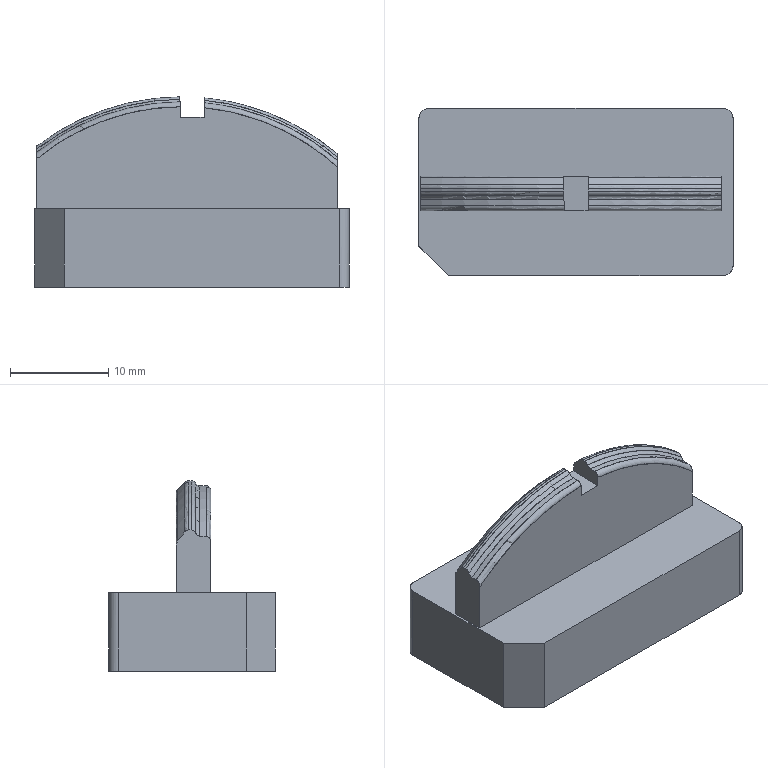NC program | PowerMill | posted with a generic post | part box 32 x 17 x 19.383 mm
Lines 1 to 1031 of 94163:
%
O0001
N104 ( POWERMILL CB  : 2026004.0)
N105 ( POST VER      : 2026.0.0.5161)
N106 ( OPTION FILE   : FANUC)
N107 ( OUTPUT WORKPLANE : WORLD)
N108 (  )
N109 ( TOOL LIST )
N110 (---------------------------------------)
N111 ( NO. | ID        | DIA.| TIP RAD|LENGTH)
N112 (---------------------------------------)
N113 (    1|D10C_1_1_1 |10.0 |  0.0   |74.84 )
N114 (    2|D4C_1_1    | 4.0 |  0.0   |66.56 )
N115 (   28|D2C_1_1    | 2.0 |  0.0   |57.36 )
N116 (    3|D10_1_1_1  |10.0 |  0.0   |74.56 )
N117 (   22|R1.5_1_1   | 3.0 |  1.5   | 64.0 )
N118 (    6|R0.5_1_1   | 1.0 |  0.5   |62.08 )
N119 (   12|D2_1_1     | 2.0 |  0.0   |57.48 )
N120 (   13|TEXT_D4_1_1| 4.0 |  0.3   |66.64 )
N121 (---------------------------------------)
N122 (  )
N123 ( NUMBER OF TOOLPATHS: 12.0 )
N124 ( ESTIMATED PROGRAM DURATION: 0 HOURS 8 MIN 19 SEC)
N125 (  )
N126 G00 G21 G80 G40 G17
N127 G90
N128 G54
N129 G53 Z0.0
N130 (---------------)
N131 ( START TOOLPATH : 精公开粗01-扫面平行-D10C )
N132 (---------------)
N133 ( TOOL NO.    :1 )
N134 ( TOOL TYPE   : ENDMILL)
N135 ( TOOL ID     : D10C_1_1_1)
N136 ( TOOL DIA    : 10.0 LENGTH 74.84)
N137 T1
N138 M6
N139 S8000 M03
N140 G00 G90 X0.0 Y0.0
N141 G43 Z10.2 H1
N142
N143 G05 P10000 R4
N144 X23.78 Y11.28
N145 Z1.133
N146 G01 Z-0.067 F6000.0
N147 X18.78 F10000.0
N148 X-18.78
N149 Y5.64
N150 X18.78
N151 Y0.0
N152 X-18.78
N153 Y-5.64
N154 X18.78
N155 Y-11.28
N156 X-18.78
N157 X-23.78
N158 G00 Z10.2
N159 G05 P0
N160 (---------------)
N161 ( END TOOLPATH : 精公开粗01-扫面平行-D10C )
N162 (---------------)
N163 ( START TOOLPATH : 精公开粗01-外形偏置-D10C )
N164 (---------------)
N165 G00 X-0.492 Y0.0 Z9.883
N166 G05 P10000 R4
N167 X-7.0152 Y16.555
N168 Z0.6943
N169 G01 Z-0.5057 F6000.0
N170 Y16.0275 F10000.0
N171 G03 X-2.2677 Y11.28 I4.7475 J0.0
N172 G01 X21.589
N173 G02 X22.589 Y10.28 I0.0 J-1.0
N174 G01 Y-0.063
N175 X16.9717 Y-0.0121
N176 X16.9358 Y-3.9737
N177 G02 X15.0976 Y-5.6289 I-1.6781 J0.0153
N178 G02 X13.6073 Y-3.6547 I0.1601 J1.6705
N179 G01 X13.9523 Y-1.7802
N180 G03 X14.0576 Y1.5627 I-10.9665 J2.0185
N181 G01 X13.7932 Y3.7726
N182 G02 X15.3061 Y5.5747 I1.6016 J0.1915
N183 G02 X17.0077 Y3.9495 I0.0887 J-1.6106
N184 G01 X16.9717 Y-0.0121
N185 X22.589 Y-0.063
N186 Y-10.28
N187 G02 X21.589 Y-11.28 I-1.0 J0.0
N188 G01 X-22.573
N189 G02 X-23.573 Y-10.28 I0.0 J1.0
N190 G01 Y10.28
N191 G02 X-22.573 Y11.28 I1.0 J0.0
N192 G01 X-2.2677
N193 X-2.0389 Y6.1703
N194 X-1.6521 Y6.1876
N195 X-0.8787 Y6.1864
N196 X-0.1053 Y6.0727
N197 X0.1278 Y6.0124
N198 X0.2294 Y5.997
N199 X0.332 Y6.0027
N200 X0.6681 Y6.0565
N201 X1.4416 Y6.0905
N202 X2.9884 Y5.9236
N203 X3.683 Y5.8007
N204 X4.5353 Y5.5786
N205 X5.3087 Y5.2734
N206 X5.7934 Y5.0273
N207 X6.0821 Y4.846
N208 X6.8214 Y4.2538
N209 X7.5071 Y3.4804
N210 X7.9833 Y2.707
N211 X8.2969 Y1.9336
N212 X8.477 Y1.1601
N213 X8.5375 Y0.3867
N214 X8.5169 Y-0.3867
N215 X8.3897 Y-1.1601
N216 X8.1319 Y-1.9336
N217 X7.7359 Y-2.707
N218 X7.1429 Y-3.4804
N219 X6.8556 Y-3.7763
N220 X6.3005 Y-4.2538
N221 X6.0821 Y-4.4062
N222 X5.3087 Y-4.834
N223 X4.8381 Y-5.0273
N224 X4.5353 Y-5.1403
N225 X3.7618 Y-5.3447
N226 X2.9884 Y-5.4861
N227 X1.4416 Y-5.6312
N228 X0.6681 Y-5.599
N229 X0.2989 Y-5.5391
N230 X0.1978 Y-5.533
N231 X0.0976 Y-5.5475
N232 X-0.1053 Y-5.5982
N233 X-0.8787 Y-5.7081
N234 X-1.6521
N235 X-3.199 Y-5.6502
N236 X-4.7458 Y-5.5156
N237 X-5.5193 Y-5.3985
N238 X-6.2927 Y-5.2201
N239 X-6.848 Y-5.0273
N240 X-7.8396 Y-4.557
N241 X-8.3012 Y-4.2538
N242 X-8.613 Y-3.9983
N243 X-9.1358 Y-3.4804
N244 X-9.7128 Y-2.707
N245 X-10.1135 Y-1.9336
N246 X-10.1935 Y-1.6892
N247 X-15.5541 Y-3.2759
N248 X-15.3948 Y-3.8142
N249 G02 X-15.861 Y-5.0171 I-1.012 J-0.2996
N250 G01 X-16.1989 Y-5.2212
N251 G02 X-17.9276 Y-4.2448 I-0.5892 J0.9753
N252 G01 X-17.9189 Y4.2871
N253 G02 X-16.4996 Y5.2423 I1.0318 J-0.001
N254 G01 X-16.0891 Y5.076
N255 G02 X-15.5129 Y3.8963 I-0.3691 J-0.9108
N256 G01 X-15.683 Y3.2983
N257 G03 X-15.6497 Y-2.9529 I10.7868 J-3.0683
N258 G01 X-15.5541 Y-3.2759
N259 X-10.1935 Y-1.6892
N260 X-10.3667 Y-1.1601
N261 X-10.4939 Y-0.3867
N262 X-10.5146 Y0.3867
N263 X-10.4537 Y1.1601
N264 X-10.2742 Y1.9336
N265 X-9.9608 Y2.707
N266 X-9.4841 Y3.4804
N267 X-8.8187 Y4.2538
N268 X-8.613 Y4.4393
N269 X-7.8396 Y4.9988
N270 X-7.0661 Y5.374
N271 X-6.2927 Y5.6588
N272 X-5.7053 Y5.8007
N273 X-4.7458 Y5.9582
N274 X-3.199 Y6.1184
N275 X-2.0389 Y6.1703
N276 X-2.2677 Y11.28
N277 G00 Z3.3056
N278 G01 X-7.0152 Y16.555
N279 G00 Z0.3056
N280 G01 Z-0.8944 F6000.0
N281 Y16.0275 F10000.0
N282 G03 X-2.2677 Y11.28 I4.7475 J0.0
N283 G01 X21.589
N284 G02 X22.589 Y10.28 I0.0 J-1.0
N285 G01 Y0.0
N286 X16.7023
N287 Y-4.6117
N288 G02 X15.9211 Y-5.3933 I-0.7816 J0.0
N289 G01 X15.5308 Y-5.3935
N290 G02 X15.0886 Y-4.6931 I-0.0003 J0.4896
N291 G01 X15.2603 Y-4.3332
N292 X15.3847 Y-4.0542
N293 X15.4944 Y-3.7692
N294 X15.5691 Y-3.5589
N295 G03 X16.0542 Y-1.5731 I-9.4775 J3.3673
N296 G01 X16.0762 Y-1.4144
N297 G03 X16.1773 Y0.7169 I-11.7057 J1.6232
N298 G01 X16.1713 Y0.8548
N299 G03 X15.7733 Y3.3476 I-10.957 J-0.4715
N300 G01 X15.7408 Y3.4633
N301 X15.5751 Y3.983
N302 X15.3737 Y4.49
N303 X15.2945 Y4.6706
N304 G02 X15.7676 Y5.3935 I0.4725 J0.207
N305 G01 X15.9216 Y5.3933
N306 G02 X16.7023 Y4.6117 I-0.0009 J-0.7816
N307 G01 Y0.0
N308 X22.589
N309 Y-10.28
N310 G02 X21.589 Y-11.28 I-1.0 J0.0
N311 G01 X-0.9179
N312 X-0.8787 Y-7.1071
N313 X-2.4256 Y-7.0926
N314 X-3.9724 Y-6.9771
N315 X-4.7458 Y-6.865
N316 X-5.9026 Y-6.5741
N317 X-6.2927 Y-6.4328
N318 X-7.0661 Y-6.0479
N319 X-7.4381 Y-5.8007
N320 X-8.0435 Y-5.3134
N321 X-8.1191 Y-5.2632
N322 X-8.2024 Y-5.2274
N323 X-8.613 Y-5.094
N324 X-9.3864 Y-4.7324
N325 X-10.1313 Y-4.2538
N326 X-10.9634 Y-3.4804
N327 X-11.5214 Y-2.707
N328 X-11.6911 Y-2.373
N329 X-17.1297 Y-4.699
N330 X-17.1126 Y-4.7532
N331 X-17.1063 Y-4.8098
N332 X-17.1039 Y-5.0207
N333 G02 X-17.6507 Y-5.0665 I-0.2751 J-0.0032
N334 G01 X-17.6834 Y-4.858
N335 G02 X-17.4208 Y-4.5238 I0.2868 J0.0449
N336 G02 X-17.1297 Y-4.699 I0.0242 J-0.2893
N337 G01 X-11.6911 Y-2.373
N338 X-11.9143 Y-1.9336
N339 X-12.1675 Y-1.1601
N340 X-12.2943 Y-0.3867
N341 X-12.3141 Y0.3867
N342 X-12.2537 Y1.1601
N343 X-12.0722 Y1.9336
N344 X-11.7609 Y2.707
N345 X-11.3025 Y3.4804
N346 X-10.9333 Y3.946
N347 X-10.6457 Y4.2538
N348 X-10.1598 Y4.6685
N349 X-9.3864 Y5.1706
N350 X-8.613 Y5.5346
N351 X-7.7473 Y5.8007
N352 X-7.0661 Y5.9571
N353 X-5.5193 Y6.2316
N354 X-4.7458 Y6.3396
N355 X-3.199 Y6.5062
N356 X-1.6521 Y6.5768
N357 X-0.8787 Y6.5746
N358 X-0.1053 Y6.4598
N359 X0.1303 Y6.3984
N360 X0.2325 Y6.3829
N361 X0.3357 Y6.3886
N362 X0.6681 Y6.442
N363 X1.4416 Y6.4769
N364 X2.215 Y6.4038
N365 X3.7618 Y6.1979
N366 X5.7592 Y5.8007
N367 X6.8556 Y5.4337
N368 X7.6165 Y5.0273
N369 X8.4024 Y4.4682
N370 X8.6389 Y4.2538
N371 X9.2959 Y3.4804
N372 X9.7444 Y2.707
N373 X10.057 Y1.9336
N374 X10.237 Y1.1601
N375 X10.2976 Y0.3867
N376 X10.2779 Y-0.3867
N377 X10.1508 Y-1.1601
N378 X9.9493 Y-1.799
N379 X9.5108 Y-2.707
N380 X9.1758 Y-3.2085
N381 X8.9556 Y-3.4804
N382 X8.4024 Y-4.0294
N383 X8.1247 Y-4.2538
N384 X7.629 Y-4.5846
N385 X6.8556 Y-4.9959
N386 X6.1948 Y-5.23
N387 X6.1125 Y-5.2679
N388 X6.0384 Y-5.32
N389 X5.4715 Y-5.8007
N390 X4.5353 Y-6.3404
N391 X3.9289 Y-6.5741
N392 X2.9884 Y-6.8119
N393 X2.215 Y-6.9477
N394 X1.4416 Y-7.027
N395 X0.6681 Y-7.0011
N396 X0.2934 Y-6.9439
N397 X0.1962 Y-6.9386
N398 X0.0998 Y-6.9523
N399 X-0.1053 Y-7.0022
N400 X-0.8787 Y-7.1071
N401 X-0.9179 Y-11.28
N402 X-22.573
N403 G02 X-23.573 Y-10.28 I0.0 J1.0
N404 G01 Y10.28
N405 G02 X-22.573 Y11.28 I1.0 J0.0
N406 G01 X-17.4129
N407 Y5.3931
N408 G02 X-17.1824 Y5.1625 I0.0 J-0.2306
N409 G02 X-17.6435 I-0.2305 J0.0
N410 G02 X-17.4129 Y5.3931 I0.2306 J0.0
N411 G01 Y11.28
N412 X-2.2677
N413 G00 Z2.9168
N414 G01 X-7.0152 Y16.555
N415 G00 Z-0.0832
N416 G01 Z-1.2832 F6000.0
N417 Y16.0275 F10000.0
N418 G03 X-2.2677 Y11.28 I4.7475 J0.0
N419 G01 X21.589
N420 G02 X22.589 Y10.28 I0.0 J-1.0
N421 G01 Y4.3674
N422 X16.8459 Y5.0753
N423 G02 X16.6917 Y4.8745 I-0.2476 J0.0305
N424 G02 X16.358 Y5.0391 I-0.0934 J0.2313
N425 G01 X16.3264 Y5.1531
N426 G02 X16.431 Y5.3816 I0.1878 J0.0521
N427 G01 X16.5044 Y5.4162
N428 G02 X16.7591 Y5.3327 I0.0833 J-0.1763
N429 G01 X16.8177 Y5.2246
N430 X16.8434 Y5.1522
N431 X16.8459 Y5.0753
N432 X22.589 Y4.3674
N433 Y-10.28
N434 G02 X21.589 Y-11.28 I-1.0 J0.0
N435 G01 X16.4647
N436 Y-6.2098
N437 G02 X15.5523 Y-5.2974 I0.0 J0.9124
N438 G02 X17.3771 I0.9124 J0.0
N439 G02 X16.4647 Y-6.2098 I-0.9124 J0.0
N440 G01 Y-11.28
N441 X1.2913
N442 X1.4416 Y-7.205
N443 X0.6681 Y-7.1765
N444 X0.1004 Y-7.079
N445 X0.0214 Y-7.0719
N446 X-0.0578 Y-7.0773
N447 X-0.8787 Y-7.1995
N448 X-3.199 Y-7.2058
N449 X-4.7458 Y-7.1718
N450 X-6.2927 Y-7.0223
N451 X-7.0661 Y-6.8746
N452 X-7.8396 Y-6.6566
N453 X-8.613 Y-6.3285
N454 X-9.3864 Y-5.8837
N455 X-10.1598 Y-5.2291
N456 X-10.3965 Y-4.9672
N457 X-10.4567 Y-4.9107
N458 X-10.5254 Y-4.8649
N459 X-10.9333 Y-4.6393
N460 X-11.7067 Y-4.075
N461 X-12.3146 Y-3.4804
N462 X-12.4801 Y-3.2781
N463 X-12.8673 Y-2.707
N464 X-13.2535 Y-1.9167
N465 X-13.5012 Y-1.1601
N466 X-13.6281 Y-0.3867
N467 X-13.645 Y0.3867
N468 X-13.5842 Y1.1601
N469 X-13.4053 Y1.9336
N470 X-13.0991 Y2.707
N471 X-12.6531 Y3.4804
N472 X-12.4801 Y3.7124
N473 X-11.9974 Y4.2538
N474 X-11.7067 Y4.5151
N475 X-11.0121 Y5.0273
N476 X-10.1598 Y5.4737
N477 X-9.3864 Y5.7609
N478 X-7.0661 Y6.3374
N479 X-5.5193 Y6.6162
N480 X-3.9724 Y6.7856
N481 X-2.4256 Y6.8418
N482 X-0.8787 Y6.8411
N483 X0.0114 Y6.6912
N484 X0.0952 Y6.6843
N485 X0.179 Y6.6915
N486 X0.6681 Y6.7755
N487 X1.4416 Y6.8135
N488 X2.9884 Y6.6914
N489 X3.7977 Y6.5741
N490 X5.3087 Y6.2848
N491 X7.2455 Y5.8007
N492 X7.629 Y5.6796
N493 X8.4024 Y5.3648
N494 X9.0101 Y5.0273
N495 X9.9493 Y4.2991
N496 X10.6532 Y3.4804
N497 X11.1056 Y2.707
N498 X11.4158 Y1.9336
N499 X11.5955 Y1.1601
N500 X11.6552 Y0.3867
N501 X11.6351 Y-0.3867
N502 X11.4961 Y-1.1935
N503 X11.2556 Y-1.9336
N504 X10.8671 Y-2.707
N505 X10.3131 Y-3.4804
N506 X9.9493 Y-3.8579
N507 X9.483 Y-4.2538
N508 X8.7548 Y-4.7437
N509 X8.5262 Y-4.8643
N510 X8.4661 Y-4.9017
N511 X8.4118 Y-4.9472
N512 X7.629 Y-5.7043
N513 X6.8556 Y-6.2071
N514 X6.0469 Y-6.5741
N515 X5.3087 Y-6.8162
N516 X4.5353 Y-6.9859
N517 X3.7618 Y-7.0891
N518 X2.9884 Y-7.1566
N519 X1.4416 Y-7.205
N520 X1.2913 Y-11.28
N521 X-22.573
N522 G02 X-23.573 Y-10.28 I0.0 J1.0
N523 G01 Y-5.5679
N524 X-18.1947
N525 G02 X-17.4546 I0.37 J0.0
N526 G02 X-18.1947 I-0.3701 J0.0
N527 G01 X-23.573
N528 Y10.28
N529 G02 X-22.573 Y11.28 I1.0 J0.0
N530 G01 X-17.9263
N531 Y5.8686
N532 G02 X-17.7089 Y5.6512 I0.0 J-0.2174
N533 G02 X-18.1437 I-0.2174 J0.0
N534 G02 X-17.9263 Y5.8686 I0.2174 J0.0
N535 G01 Y11.28
N536 X-2.2677
N537 G00 Z2.5281
N538 G01 X-7.0152 Y16.555
N539 G00 Z-0.4719
N540 G01 Z-1.6719 F6000.0
N541 Y16.0275 F10000.0
N542 G03 X-2.2677 Y11.28 I4.7475 J0.0
N543 G01 X21.589
N544 G02 X22.589 Y10.28 I0.0 J-1.0
N545 G01 Y4.2803
N546 X18.089
N547 X22.589
N548 Y-4.0539
N549 X18.089
N550 X22.589
N551 Y-10.28
N552 G02 X21.589 Y-11.28 I-1.0 J0.0
N553 G01 X4.1906
N554 X4.0519 Y-7.1981
N555 X3.7618 Y-7.208
N556 X1.4416 Y-7.2096
N557 X0.6681 Y-7.1789
N558 X0.096 Y-7.0804
N559 X0.017 Y-7.0732
N560 X-0.0621 Y-7.0786
N561 X-0.8787 Y-7.1996
N562 X-1.0358 Y-7.1999
N563 X-3.199 Y-7.2057
N564 X-3.2468 Y-7.2047
N565 X-5.5193 Y-7.2096
N566 X-7.0661 Y-7.146
N567 X-7.8396 Y-7.0488
N568 X-8.613 Y-6.8818
N569 X-9.3864 Y-6.6519
N570 X-10.1598 Y-6.2979
N571 X-10.9333 Y-5.8302
N572 X-11.7067 Y-5.1502
N573 X-12.1156 Y-4.6481
N574 X-12.1628 Y-4.5976
N575 X-12.2166 Y-4.5542
N576 X-12.4801 Y-4.3697
N577 X-13.2535 Y-3.6872
N578 X-13.4442 Y-3.4804
N579 X-13.9984 Y-2.707
N580 X-14.3703 Y-1.9336
N581 X-14.6196 Y-1.1601
N582 X-14.7464 Y-0.3867
N583 X-14.7667 Y0.3867
N584 X-14.7064 Y1.1601
N585 X-14.5263 Y1.9336
N586 X-14.2283 Y2.707
N587 X-14.1489 Y2.8579
N588 X-18.1306 Y4.9545
N589 X-14.1489 Y2.8579
N590 X-14.027 Y3.0894
N591 X-13.7845 Y3.4804
N592 X-13.2535 Y4.1271
N593 X-12.4801 Y4.807
N594 X-12.1668 Y5.0273
N595 X-11.7067 Y5.2921
N596 X-10.9333 Y5.6423
N597 X-9.3864 Y6.1271
N598 X-7.7021 Y6.5741
N599 X-7.0661 Y6.6894
N600 X-6.2927 Y6.7901
N601 X-5.5193 Y6.8484
N602 X-4.7458 Y6.8679
N603 X-0.8787 Y6.8574
N604 X-0.068 Y6.7297
N605 X0.0152 Y6.7236
N606 X0.0982 Y6.7315
N607 X0.6681 Y6.8338
N608 X1.4416 Y6.8743
N609 X2.215
N610 X3.7618 Y6.833
N611 X4.5353 Y6.7675
N612 X5.7064 Y6.5741
N613 X6.8556 Y6.278
N614 X8.4455 Y5.8007
N615 X9.1758 Y5.54
N616 X9.9493 Y5.1574
N617 X10.1628 Y5.0273
N618 X10.7227 Y4.6102
N619 X11.1265 Y4.2538
N620 X11.4961 Y3.8541
N621 X11.782 Y3.4804
N622 X12.2278 Y2.707
N623 X12.5368 Y1.9336
N624 X12.7162 Y1.1601
N625 X12.776 Y0.3867
N626 X12.7585 Y-0.3867
N627 X12.6317 Y-1.1601
N628 X12.3795 Y-1.9336
N629 X11.995 Y-2.707
N630 X11.4961 Y-3.4161
N631 X10.7227 Y-4.1732
N632 X10.2319 Y-4.5404
N633 X10.1819 Y-4.5832
N634 X10.138 Y-4.6322
N635 X9.828 Y-5.0273
N636 X9.1758 Y-5.649
N637 X8.9857 Y-5.8007
N638 X8.4024 Y-6.1714
N639 X7.5902 Y-6.5741
N640 X6.8556 Y-6.8173
N641 X6.0821 Y-7.0074
N642 X5.3087 Y-7.1194
N643 X4.5353 Y-7.1817
N644 X4.0519 Y-7.1981
N645 X4.1906 Y-11.28
N646 X-22.573
N647 G02 X-23.573 Y-10.28 I0.0 J1.0
N648 G01 Y-5.5057
N649 X-19.073
N650 X-23.573
N651 Y10.28
N652 G02 X-22.573 Y11.28 I1.0 J0.0
N653 G01 X-2.2677
N654 G00 Z2.1394
N655 G01 X-7.0152 Y16.555
N656 G00 Z-0.8606
N657 G01 Z-2.0606 F6000.0
N658 Y16.0275 F10000.0
N659 G03 X-2.2677 Y11.28 I4.7475 J0.0
N660 G01 X21.589
N661 G02 X22.589 Y10.28 I0.0 J-1.0
N662 G01 Y5.1213
N663 X18.089
N664 X22.589
N665 Y-5.4771
N666 X18.089
N667 X22.589
N668 Y-10.28
N669 G02 X21.589 Y-11.28 I-1.0 J0.0
N670 G01 X6.2443
N671 X6.0821 Y-7.1789
N672 X5.3087 Y-7.2095
N673 X1.4416 Y-7.2096
N674 X0.6681 Y-7.1792
N675 X0.0961 Y-7.0805
N676 X0.017 Y-7.0732
N677 X-0.0623 Y-7.0786
N678 X-0.8787 Y-7.1996
N679 X-1.0316 Y-7.1998
N680 X-1.0358 Y-7.1999
N681 X-3.199 Y-7.2057
N682 X-3.2468 Y-7.2046
N683 X-5.5193 Y-7.2095
N684 X-5.5765 Y-7.2072
N685 X-7.0661 Y-7.2096
N686 X-7.8396 Y-7.1897
N687 X-8.613 Y-7.1337
N688 X-9.3864 Y-7.0073
N689 X-10.1598 Y-6.8023
N690 X-10.8146 Y-6.5741
N691 X-11.7067 Y-6.1013
N692 X-12.1618 Y-5.8007
N693 X-12.4801 Y-5.5443
N694 X-13.0025 Y-5.0273
N695 X-13.502 Y-4.3539
N696 X-14.027 Y-3.8946
N697 X-14.4273 Y-3.4804
N698 X-14.8004 Y-2.9881
N699 X-14.9796 Y-2.707
N700 X-15.3559 Y-1.9336
N701 X-15.5738 Y-1.2866
N702 X-15.7328 Y-0.3867
N703 X-15.7535 Y0.3867
N704 X-15.693 Y1.1601
N705 X-15.5125 Y1.9336
N706 X-15.2093 Y2.707
N707 X-14.8004 Y3.4253
N708 X-14.1115 Y4.2538
N709 X-13.2535 Y4.969
N710 X-12.4801 Y5.4114
N711 X-11.7067 Y5.7325
N712 X-10.9333 Y6.0101
N713 X-9.3864 Y6.4999
N714 X-8.613 Y6.6853
N715 X-7.8396 Y6.7939
N716 X-7.0661 Y6.8552
N717 X-6.2927 Y6.8744
N718 X-0.8787 Y6.8613
N719 X-0.0701 Y6.7303
N720 X0.0159 Y6.7239
N721 X0.1017 Y6.7324
N722 X0.6681 Y6.8384
N723 X1.4416 Y6.8743
N724 X1.4931
N725 X2.215
N726 X2.2444 Y6.8735
N727 X4.5353 Y6.8711
N728 X5.3087 Y6.8445
N729 X6.0821 Y6.7673
N730 X7.1074 Y6.5741
N731 X8.4024 Y6.1809
N732 X9.9493 Y5.643
N733 X10.7227 Y5.2843
N734 X11.1653 Y5.0273
N735 X11.4961 Y4.7936
N736 X12.2695 Y4.0887
N737 X12.7649 Y3.4804
N738 X13.043 Y3.0278
N739 X13.2083 Y2.707
N740 X13.5011 Y1.9336
N741 X13.6803 Y1.1601
N742 X13.7405 Y0.3867
N743 X13.721 Y-0.3867
N744 X13.5942 Y-1.1601
N745 X13.3504 Y-1.9336
N746 X13.043 Y-2.5921
N747 X12.4261 Y-3.4804
N748 X12.2695 Y-3.6505
N749 X11.4961 Y-4.3648
N750 X11.003 Y-5.0273
N751 X10.7227 Y-5.3245
N752 X10.1635 Y-5.8007
N753 X9.9493 Y-5.9527
N754 X9.1758 Y-6.408
N755 X8.8184 Y-6.5741
N756 X8.4024 Y-6.7272
N757 X7.629 Y-6.9554
N758 X6.8556 Y-7.0957
N759 X6.0821 Y-7.1789
N760 X6.2443 Y-11.28
N761 X-22.573
N762 G02 X-23.573 Y-10.28 I0.0 J1.0
N763 G01 Y10.28
N764 G02 X-22.573 Y11.28 I1.0 J0.0
N765 G01 X-2.2677
N766 G00 Z1.7507
N767 G01 X-7.0152 Y16.555
N768 G00 Z-1.2493
N769 G01 Z-2.4493 F6000.0
N770 Y16.0275 F10000.0
N771 G03 X-2.2677 Y11.28 I4.7475 J0.0
N772 G01 X21.589
N773 G02 X22.589 Y10.28 I0.0 J-1.0
N774 G01 Y-10.28
N775 G02 X21.589 Y-11.28 I-1.0 J0.0
N776 G01 X7.2217
N777 X6.9522 Y-7.1938
N778 X6.8556 Y-7.2001
N779 X6.0821 Y-7.2096
N780 X4.6377 Y-7.2094
N781 X1.4416 Y-7.2095
N782 X1.4292 Y-7.2091
N783 X-4.9822 Y-7.2083
N784 X-5.5193 Y-7.2095
N785 X-5.549 Y-7.2083
N786 X-6.2287 Y-7.2082
N787 X-7.0661 Y-7.2095
N788 X-7.1227 Y-7.2081
N789 X-8.613 Y-7.2079
N790 X-9.3864 Y-7.1716
N791 X-10.1598 Y-7.0669
N792 X-10.9333 Y-6.9
N793 X-11.7067 Y-6.6322
N794 X-12.4801 Y-6.2625
N795 X-13.1696 Y-5.8007
N796 X-14.0078 Y-5.0273
N797 X-14.5683 Y-4.2538
N798 X-15.3054 Y-3.4804
N799 X-15.5738 Y-3.1386
N800 X-15.8577 Y-2.707
N801 X-16.2283 Y-1.9336
N802 X-16.4731 Y-1.1601
N803 X-16.6 Y-0.3867
N804 X-16.619 Y0.3867
N805 X-16.5583 Y1.1601
N806 X-16.3794 Y1.9336
N807 X-16.0838 Y2.707
N808 X-15.643 Y3.4804
N809 X-14.9908 Y4.2538
N810 X-14.8004 Y4.4449
N811 X-14.0586 Y5.0273
N812 X-13.2535 Y5.4775
N813 X-12.4749 Y5.8007
N814 X-10.9333 Y6.374
N815 X-10.2734 Y6.5741
N816 X-9.3864 Y6.7579
N817 X-8.613 Y6.8449
N818 X-7.8396 Y6.8743
N819 X-6.2948
N820 X-6.2927
N821 X-6.2718
N822 X5.3087 Y6.8744
N823 X6.0821 Y6.867
N824 X6.8556 Y6.8252
N825 X7.629 Y6.7185
N826 X8.2703 Y6.5741
N827 X9.1758 Y6.2861
N828 X10.7227 Y5.7026
N829 X11.4961 Y5.3539
N830 X12.2695 Y4.8815
N831 X12.9941 Y4.2538
N832 X13.6405 Y3.4804
N833 X13.8164 Y3.208
N834 X14.0856 Y2.707
N835 X14.3805 Y1.9336
N836 X14.56 Y1.1601
N837 X14.6206 Y0.3867
N838 X14.6002 Y-0.3867
N839 X14.4735 Y-1.1601
N840 X14.2287 Y-1.9336
N841 X13.8553 Y-2.707
N842 X13.5142 Y-3.1866
N843 X17.1815 Y-5.7945
N844 X13.5142 Y-3.1866
N845 X13.3053 Y-3.4804
N846 X12.6183 Y-4.1719
N847 X12.5908 Y-4.2137
N848 X12.2695 Y-4.7011
N849 X12.0086 Y-5.0273
N850 X11.4961 Y-5.538
N851 X11.171 Y-5.8007
N852 X10.7227 Y-6.1152
N853 X9.8537 Y-6.5741
N854 X9.1758 Y-6.8241
N855 X8.4024 Y-7.0214
N856 X7.629 Y-7.1491
N857 X6.9522 Y-7.1938
N858 X7.2217 Y-11.28
N859 X-22.573
N860 G02 X-23.573 Y-10.28 I0.0 J1.0
N861 G01 Y10.28
N862 G02 X-22.573 Y11.28 I1.0 J0.0
N863 G01 X-2.2677
N864 G00 Z1.3619
N865 G01 X-7.0152 Y16.555
N866 G00 Z-1.6381
N867 G01 Z-2.8381 F6000.0
N868 Y16.0275 F10000.0
N869 G03 X-2.2677 Y11.28 I4.7475 J0.0
N870 G01 X21.589
N871 G02 X22.589 Y10.28 I0.0 J-1.0
N872 G01 Y-10.28
N873 G02 X21.589 Y-11.28 I-1.0 J0.0
N874 G01 X7.6291
N875 X7.629 Y-7.2092
N876 X6.1049 Y-7.2093
N877 X6.0821 Y-7.2095
N878 X4.6377 Y-7.2094
N879 X1.4416 Y-7.2095
N880 X1.4381 Y-7.2094
N881 X-9.3864 Y-7.2096
N882 X-10.1598 Y-7.1844
N883 X-10.9333 Y-7.1073
N884 X-11.7067 Y-6.9462
N885 X-12.4801 Y-6.6923
N886 X-13.2535 Y-6.3409
N887 X-14.027 Y-5.8295
N888 X-14.8004 Y-5.1317
N889 X-15.4552 Y-4.2538
N890 X-15.5462 Y-4.0915
N891 X-15.584 Y-4.0336
N892 X-15.6295 Y-3.9816
N893 X-15.8463 Y-3.7656
N894 X-16.3472 Y-3.1793
N895 X-16.6579 Y-2.707
N896 X-17.0287 Y-1.9336
N897 X-17.2661 Y-1.1601
N898 X-17.3927 Y-0.3867
N899 X-17.4103 Y0.3867
N900 X-17.3501 Y1.1601
N901 X-17.173 Y1.9336
N902 X-16.8861 Y2.707
N903 X-16.4435 Y3.4804
N904 X-15.7983 Y4.2538
N905 X-15.5738 Y4.4743
N906 X-14.8658 Y5.0273
N907 X-14.027 Y5.4986
N908 X-12.4801 Y6.1556
N909 X-11.7067 Y6.4475
N910 X-10.9333 Y6.6662
N911 X-10.1598 Y6.7981
N912 X-9.3864 Y6.8602
N913 X-8.613 Y6.8743
N914 X-6.2931
N915 X-6.2927
N916 X-6.2885
N917 X6.8556 Y6.8744
N918 X7.629 Y6.8496
N919 X8.4024 Y6.7608
N920 X9.1758 Y6.6027
N921 X9.9493 Y6.365
N922 X10.7227 Y6.0561
N923 X12.2695 Y5.3745
N924 X13.043 Y4.9055
N925 X13.7997 Y4.2538
N926 X14.4443 Y3.4804
N927 X14.5898 Y3.2568
N928 X14.8874 Y2.707
N929 X15.1748 Y1.9336
N930 X15.3528 Y1.1601
N931 X15.4101 Y0.3867
N932 X15.3944 Y-0.3867
N933 X15.2679 Y-1.1601
N934 X15.0292 Y-1.9336
N935 X14.6588 Y-2.707
N936 X14.1063 Y-3.4804
N937 X13.6257 Y-3.9817
N938 X13.5848 Y-4.0301
N939 X13.5504 Y-4.0833
N940 X13.4548 Y-4.2538
N941 X12.895 Y-5.0273
N942 X12.2695 Y-5.6338
N943 X11.4961 Y-6.2012
N944 X10.7683 Y-6.5741
N945 X9.9493 Y-6.8803
N946 X9.1758 Y-7.0613
N947 X8.4024 Y-7.1704
N948 X7.629 Y-7.2092
N949 X7.6291 Y-11.28
N950 X-22.573
N951 G02 X-23.573 Y-10.28 I0.0 J1.0
N952 G01 Y10.28
N953 G02 X-22.573 Y11.28 I1.0 J0.0
N954 G01 X-2.2677
N955 G00 Z0.9732
N956 G01 X-7.0152 Y16.555
N957 G00 Z-2.0268
N958 G01 Z-3.2268 F6000.0
N959 Y16.0275 F10000.0
N960 G03 X-2.2677 Y11.28 I4.7475 J0.0
N961 G01 X21.589
N962 G02 X22.589 Y10.28 I0.0 J-1.0
N963 G01 Y-10.28
N964 G02 X21.589 Y-11.28 I-1.0 J0.0
N965 G01 X-0.8787
N966 Y-7.2096
N967 X-10.1598
N968 X-10.9333 Y-7.1929
N969 X-11.7067 Y-7.1225
N970 X-12.4801 Y-6.9675
N971 X-13.2535 Y-6.7237
N972 X-14.027 Y-6.3682
N973 X-14.886 Y-5.8007
N974 X-15.6986 Y-5.0273
N975 X-16.2587 Y-4.2538
N976 X-16.4258 Y-3.9438
N977 X-16.4621 Y-3.8863
N978 X-16.5059 Y-3.8342
N979 X-16.5648 Y-3.773
N980 X-17.1207 Y-3.0977
N981 X-17.3754 Y-2.707
N982 X-17.7464 Y-1.9336
N983 X-17.9821 Y-1.1601
N984 X-18.1087 Y-0.3867
N985 X-18.1305 Y0.3867
N986 X-18.0702 Y1.1601
N987 X-17.8941 Y1.9299
N988 X-17.6063 Y2.707
N989 X-17.1631 Y3.4804
N990 X-16.5257 Y4.2538
N991 X-16.3472 Y4.4311
N992 X-15.5915 Y5.0273
N993 X-14.8004 Y5.4801
N994 X-14.1212 Y5.8007
N995 X-12.4801 Y6.4811
N996 X-11.7067 Y6.6951
N997 X-10.9333 Y6.8188
N998 X-10.1598 Y6.87
N999 X-9.3864 Y6.8744
N1000 X7.629
N1001 X8.4024 Y6.859
N1002 X9.1758 Y6.7867
N1003 X9.9493 Y6.6387
N1004 X10.7227 Y6.4019
N1005 X12.2695 Y5.7339
N1006 X13.043 Y5.3613
N1007 X13.8164 Y4.8703
N1008 X14.5241 Y4.2538
N1009 X15.1617 Y3.4804
N1010 X15.3632 Y3.1637
N1011 X15.6042 Y2.707
N1012 X15.8979 Y1.9336
N1013 X16.0754 Y1.1601
N1014 X16.1354 Y0.3867
N1015 X16.1157 Y-0.3867
N1016 X15.9891 Y-1.1601
N1017 X15.7446 Y-1.9336
N1018 X15.3729 Y-2.707
N1019 X14.8216 Y-3.4804
N1020 X14.4991 Y-3.8369
N1021 X14.4615 Y-3.8838
N1022 X14.4299 Y-3.9348
N1023 X14.2577 Y-4.2538
N1024 X13.6992 Y-5.0273
N1025 X12.8854 Y-5.8007
N1026 X12.2695 Y-6.2304
N1027 X11.5982 Y-6.5741
N1028 X10.7227 Y-6.9042
N1029 X9.9493 Y-7.0821
N1030 X9.1758 Y-7.1771
N1031 X8.4024 Y-7.2096
N1032 X-0.8787
N1033 Y-11.28
N1034 X-22.573
N1035 G02 X-23.573 Y-10.28 I0.0 J1.0
N1036 G01 Y10.28
N1037 G02 X-22.573 Y11.28 I1.0 J0.0
N1038 G01 X-2.2677
N1039 G00 Z0.5845
N1040 G01 X-7.0152 Y16.555
N1041 G00 Z-2.4155
N1042 G01 Z-3.6155 F6000.0
N1043 Y16.0275 F10000.0
N1044 G03 X-2.2677 Y11.28 I4.7475 J0.0
N1045 G01 X21.589
N1046 G02 X22.589 Y10.28 I0.0 J-1.0
N1047 G01 Y-10.28
N1048 G02 X21.589 Y-11.28 I-1.0 J0.0
N1049 G01 X-0.8787
N1050 Y-7.2096
N1051 X-10.9333
N1052 X-11.7067 Y-7.1957
N1053 X-12.4801 Y-7.1246
N1054 X-13.2535 Y-6.9664
N1055 X-14.027 Y-6.7212
N1056 X-14.8004 Y-6.361
N1057 X-15.5738 Y-5.856
N1058 X-16.3472 Y-5.1341
N1059 X-17.0007 Y-4.2538
N1060 X-17.2334 Y-3.8077
N1061 X-17.2625 Y-3.7588
N1062 X-17.297 Y-3.7136
N1063 X-17.4969 Y-3.4804
N1064 X-17.8941 Y-2.9504
N1065 X-18.0461 Y-2.707
N1066 X-18.4168 Y-1.9336
N1067 X-18.6513 Y-1.1601
N1068 X-18.7778 Y-0.3867
N1069 X-18.7974 Y0.3867
N1070 X-18.7372 Y1.1601
N1071 X-18.5616 Y1.9336
N1072 X-18.275 Y2.707
N1073 X-17.8941 Y3.3865
N1074 X-17.2021 Y4.2538
N1075 X-16.3472 Y4.977
N1076 X-15.5738 Y5.4454
N1077 X-14.027 Y6.1912
N1078 X-13.2535 Y6.4957
N1079 X-12.4801 Y6.7038
N1080 X-11.7067 Y6.8268
N1081 X-10.9333 Y6.8729
N1082 X-9.6211 Y6.873
N1083 X-9.3864 Y6.8743
N1084 X7.629
N1085 X7.6293
N1086 X8.4024 Y6.8744
N1087 X9.1758 Y6.8639
N1088 X9.9493 Y6.7974
N1089 X10.7227 Y6.6491
N1090 X11.4961 Y6.4092
N1091 X12.2695 Y6.0789
N1092 X13.8164 Y5.3124
N1093 X14.5898 Y4.8012
N1094 X15.2033 Y4.2538
N1095 X15.8314 Y3.4804
N1096 X16.1367 Y2.9816
N1097 X16.2748 Y2.707
N1098 X16.5622 Y1.9336
N1099 X16.7354 Y1.1601
N1100 X16.7954 Y0.3867
N1101 X16.7767 Y-0.3867
N1102 X16.6502 Y-1.1601
N1103 X16.4167 Y-1.9336
N1104 X16.0457 Y-2.707
N1105 X15.4982 Y-3.4804
N1106 X15.2984 Y-3.7127
N1107 X15.2635 Y-3.7582
N1108 X15.2342 Y-3.8075
N1109 X15.0012 Y-4.2538
N1110 X14.5898 Y-4.8485
N1111 X14.441 Y-5.0273
N1112 X13.6425 Y-5.8007
N1113 X13.043 Y-6.2236
N1114 X12.3663 Y-6.5741
N1115 X11.4961 Y-6.9018
N1116 X10.7227 Y-7.0839
N1117 X9.9493 Y-7.1787
N1118 X9.1758 Y-7.2096
N1119 X-0.8787
N1120 Y-11.28
N1121 X-22.573
N1122 G02 X-23.573 Y-10.28 I0.0 J1.0
N1123 G01 Y10.28
N1124 G02 X-22.573 Y11.28 I1.0 J0.0
N1125 G01 X-2.2677
N1126 G00 Z0.1958
N1127 G01 X-7.0152 Y16.555
N1128 G00 Z-2.8042